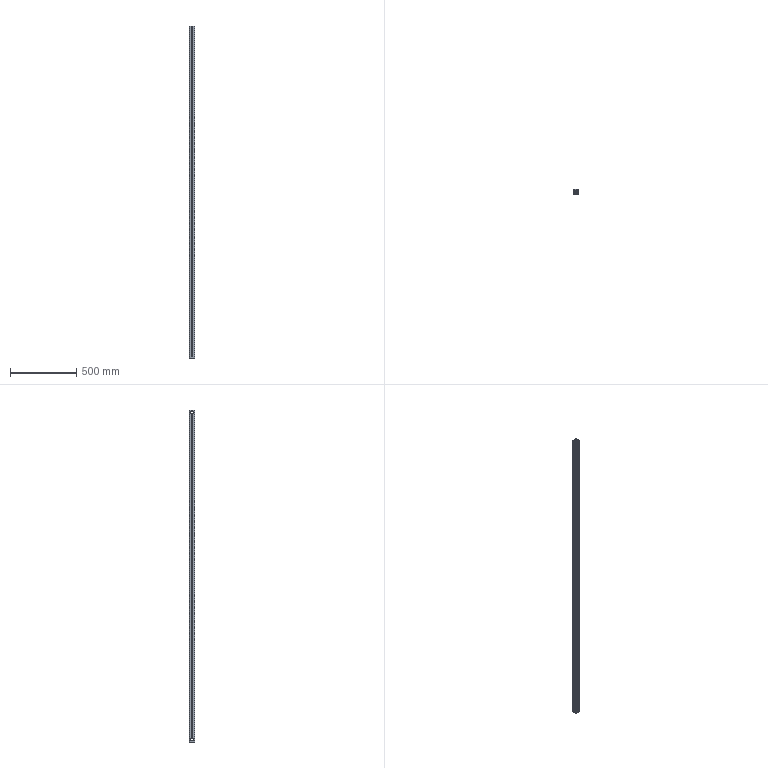Part | SolidWorks | features BaseBody 1, HoleWzd 1, MoveFace 1 | 1 solid | 242 faces | box 40 x 40 x 2500 mm | volume 1471799 mm3 | plane 187 | cylinder 55 | commonest cylinder face diameters 6.8 x15 2 x14 19 x12 1 x6 5 x4 9 x4